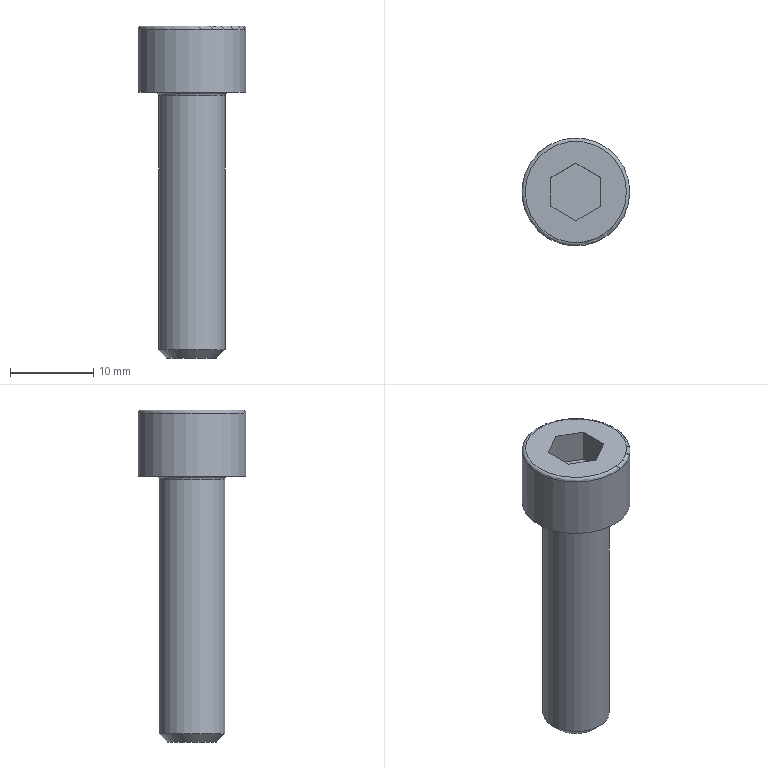Part | STEP file | solid 162 | 1 solid | 15 faces | box 13 x 13 x 40 mm | volume 2534 mm3 | plane 10 | cylinder 2 | torus 2 | cone 1 | commonest cylinder face diameters 8 x1 13 x1